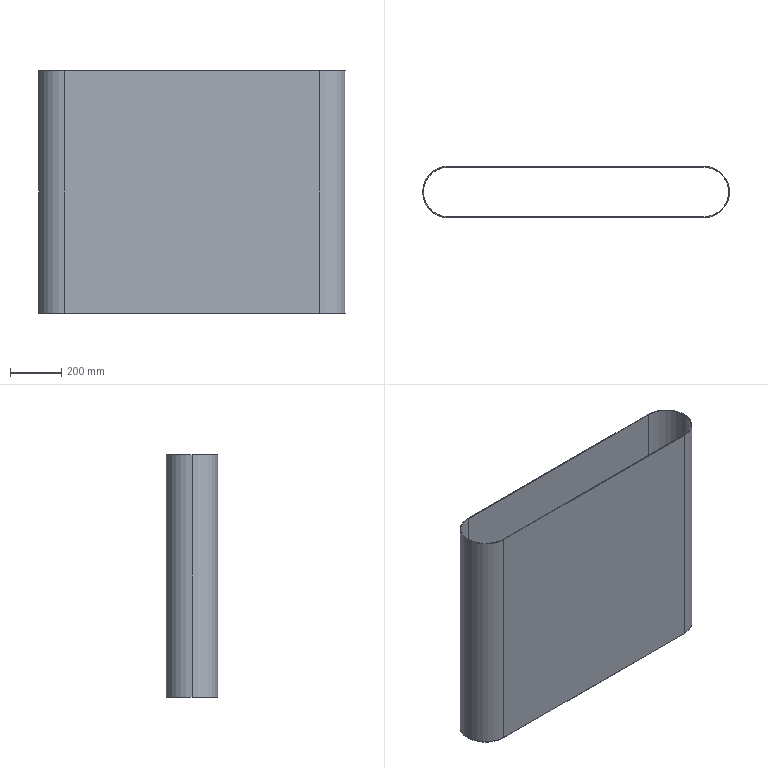Part | STEP file | Belt XG | 1 solid | 12 faces | box 1201 x 201 x 950 mm | volume 7472801 mm3 | cylinder 6 | plane 6 | commonest cylinder face diameters 195 x3 201 x3
STEP:
#1=CARTESIAN_POINT('',(0.,0.,0.));
#2=DIRECTION('',(0.,0.,1.));
#3=DIRECTION('',(1.,0.,0.));
#4=AXIS2_PLACEMENT_3D('',#1,#2,#3);
#5=CARTESIAN_POINT('',(-500.,97.5,475.));
#6=VERTEX_POINT('',#5);
#7=CARTESIAN_POINT('',(-500.,97.5,-475.));
#8=VERTEX_POINT('',#7);
#9=CARTESIAN_POINT('',(-500.,97.5,475.));
#10=DIRECTION('',(0.,0.,-1.));
#11=VECTOR('',#10,1.);
#12=LINE('',#9,#11);
#13=CARTESIAN_POINT('',(-500.,0.,475.));
#14=DIRECTION('',(0.,0.,-1.));
#15=DIRECTION('',(-1.,0.,0.));
#16=AXIS2_PLACEMENT_3D('',#13,#14,#15);
#17=CYLINDRICAL_SURFACE('',#16,97.5);
#18=CARTESIAN_POINT('',(1.571,0.));
#19=DIRECTION('',(0.,1.));
#20=VECTOR('',#19,1.);
#21=LINE('',#18,#20);
#22=(GEOMETRIC_REPRESENTATION_CONTEXT(2)PARAMETRIC_REPRESENTATION_CONTEXT()REPRESENTATION_CONTEXT('',''));
#23=DEFINITIONAL_REPRESENTATION('',(#21),#22);
#24=PCURVE('',#17,#23);
#25=CARTESIAN_POINT('',(-500.,97.5,475.));
#26=DIRECTION('',(0.,-1.,0.));
#27=DIRECTION('',(0.,0.,-1.));
#28=AXIS2_PLACEMENT_3D('',#25,#26,#27);
#29=PLANE('',#28);
#30=CARTESIAN_POINT('',(0.,0.));
#31=DIRECTION('',(1.,0.));
#32=VECTOR('',#31,1.);
#33=LINE('',#30,#32);
#34=(GEOMETRIC_REPRESENTATION_CONTEXT(2)PARAMETRIC_REPRESENTATION_CONTEXT()REPRESENTATION_CONTEXT('',''));
#35=DEFINITIONAL_REPRESENTATION('',(#33),#34);
#36=PCURVE('',#29,#35);
#37=SURFACE_CURVE('',#12,(#24,#36),.PCURVE_S1.);
#38=EDGE_CURVE('',#6,#8,#37,.T.);
#39=ORIENTED_EDGE('',*,*,#38,.T.);
#40=CARTESIAN_POINT('',(-597.5,0.,-475.));
#41=VERTEX_POINT('',#40);
#42=CARTESIAN_POINT('',(-500.,0.,-475.));
#43=DIRECTION('',(0.,0.,1.));
#44=DIRECTION('',(1.,0.,0.));
#45=AXIS2_PLACEMENT_3D('',#42,#43,#44);
#46=CIRCLE('',#45,97.5);
#47=CARTESIAN_POINT('',(3.142,950.));
#48=DIRECTION('',(-1.,0.));
#49=VECTOR('',#48,1.);
#50=LINE('',#47,#49);
#51=(GEOMETRIC_REPRESENTATION_CONTEXT(2)PARAMETRIC_REPRESENTATION_CONTEXT()REPRESENTATION_CONTEXT('',''));
#52=DEFINITIONAL_REPRESENTATION('',(#50),#51);
#53=PCURVE('',#17,#52);
#54=CARTESIAN_POINT('',(-500.,0.,-475.));
#55=DIRECTION('',(0.,0.,1.));
#56=DIRECTION('',(1.,0.,0.));
#57=AXIS2_PLACEMENT_3D('',#54,#55,#56);
#58=PLANE('',#57);
#59=CARTESIAN_POINT('',(0.,0.));
#60=DIRECTION('',(1.,0.));
#61=AXIS2_PLACEMENT_2D('',#59,#60);
#62=CIRCLE('',#61,97.5);
#63=(GEOMETRIC_REPRESENTATION_CONTEXT(2)PARAMETRIC_REPRESENTATION_CONTEXT()REPRESENTATION_CONTEXT('',''));
#64=DEFINITIONAL_REPRESENTATION('',(#62),#63);
#65=PCURVE('',#58,#64);
#66=SURFACE_CURVE('',#46,(#53,#65),.PCURVE_S1.);
#67=EDGE_CURVE('',#8,#41,#66,.T.);
#68=ORIENTED_EDGE('',*,*,#67,.T.);
#69=CARTESIAN_POINT('',(-597.5,0.,475.));
#70=VERTEX_POINT('',#69);
#71=CARTESIAN_POINT('',(-597.5,0.,475.));
#72=DIRECTION('',(0.,0.,-1.));
#73=VECTOR('',#72,1.);
#74=LINE('',#71,#73);
#75=CARTESIAN_POINT('',(0.,0.));
#76=DIRECTION('',(0.,1.));
#77=VECTOR('',#76,1.);
#78=LINE('',#75,#77);
#79=(GEOMETRIC_REPRESENTATION_CONTEXT(2)PARAMETRIC_REPRESENTATION_CONTEXT()REPRESENTATION_CONTEXT('',''));
#80=DEFINITIONAL_REPRESENTATION('',(#78),#79);
#81=PCURVE('',#17,#80);
#82=CARTESIAN_POINT('',(-500.,0.,475.));
#83=DIRECTION('',(0.,0.,-1.));
#84=DIRECTION('',(-1.,0.,0.));
#85=AXIS2_PLACEMENT_3D('',#82,#83,#84);
#86=CYLINDRICAL_SURFACE('',#85,97.5);
#87=CARTESIAN_POINT('',(6.283,0.));
#88=DIRECTION('',(0.,1.));
#89=VECTOR('',#88,1.);
#90=LINE('',#87,#89);
#91=(GEOMETRIC_REPRESENTATION_CONTEXT(2)PARAMETRIC_REPRESENTATION_CONTEXT()REPRESENTATION_CONTEXT('',''));
#92=DEFINITIONAL_REPRESENTATION('',(#90),#91);
#93=PCURVE('',#86,#92);
#94=SURFACE_CURVE('',#74,(#81,#93),.PCURVE_S1.);
#95=EDGE_CURVE('',#70,#41,#94,.T.);
#96=ORIENTED_EDGE('',*,*,#95,.F.);
#97=CARTESIAN_POINT('',(-500.,0.,475.));
#98=DIRECTION('',(0.,0.,1.));
#99=DIRECTION('',(1.,0.,0.));
#100=AXIS2_PLACEMENT_3D('',#97,#98,#99);
#101=CIRCLE('',#100,97.5);
#102=CARTESIAN_POINT('',(3.142,0.));
#103=DIRECTION('',(-1.,0.));
#104=VECTOR('',#103,1.);
#105=LINE('',#102,#104);
#106=(GEOMETRIC_REPRESENTATION_CONTEXT(2)PARAMETRIC_REPRESENTATION_CONTEXT()REPRESENTATION_CONTEXT('',''));
#107=DEFINITIONAL_REPRESENTATION('',(#105),#106);
#108=PCURVE('',#17,#107);
#109=CARTESIAN_POINT('',(-500.,0.,475.));
#110=DIRECTION('',(0.,0.,1.));
#111=DIRECTION('',(1.,0.,0.));
#112=AXIS2_PLACEMENT_3D('',#109,#110,#111);
#113=PLANE('',#112);
#114=CARTESIAN_POINT('',(0.,0.));
#115=DIRECTION('',(1.,0.));
#116=AXIS2_PLACEMENT_2D('',#114,#115);
#117=CIRCLE('',#116,97.5);
#118=(GEOMETRIC_REPRESENTATION_CONTEXT(2)PARAMETRIC_REPRESENTATION_CONTEXT()REPRESENTATION_CONTEXT('',''));
#119=DEFINITIONAL_REPRESENTATION('',(#117),#118);
#120=PCURVE('',#113,#119);
#121=SURFACE_CURVE('',#101,(#108,#120),.PCURVE_S1.);
#122=EDGE_CURVE('',#6,#70,#121,.T.);
#123=ORIENTED_EDGE('',*,*,#122,.F.);
#124=EDGE_LOOP('',(#39,#68,#96,#123));
#125=FACE_BOUND('',#124,.F.);
#126=ADVANCED_FACE('',(#125),#17,.F.);
#127=CARTESIAN_POINT('',(-600.5,0.,475.));
#128=VERTEX_POINT('',#127);
#129=CARTESIAN_POINT('',(-500.,-100.5,475.));
#130=VERTEX_POINT('',#129);
#131=CARTESIAN_POINT('',(-500.,0.,475.));
#132=DIRECTION('',(0.,0.,1.));
#133=DIRECTION('',(1.,0.,0.));
#134=AXIS2_PLACEMENT_3D('',#131,#132,#133);
#135=CIRCLE('',#134,100.5);
#136=CARTESIAN_POINT('',(-500.,0.,475.));
#137=DIRECTION('',(0.,0.,-1.));
#138=DIRECTION('',(-1.,0.,0.));
#139=AXIS2_PLACEMENT_3D('',#136,#137,#138);
#140=CYLINDRICAL_SURFACE('',#139,100.5);
#141=CARTESIAN_POINT('',(9.425,0.));
#142=DIRECTION('',(-1.,0.));
#143=VECTOR('',#142,1.);
#144=LINE('',#141,#143);
#145=(GEOMETRIC_REPRESENTATION_CONTEXT(2)PARAMETRIC_REPRESENTATION_CONTEXT()REPRESENTATION_CONTEXT('',''));
#146=DEFINITIONAL_REPRESENTATION('',(#144),#145);
#147=PCURVE('',#140,#146);
#148=CARTESIAN_POINT('',(0.,0.));
#149=DIRECTION('',(1.,0.));
#150=AXIS2_PLACEMENT_2D('',#148,#149);
#151=CIRCLE('',#150,100.5);
#152=(GEOMETRIC_REPRESENTATION_CONTEXT(2)PARAMETRIC_REPRESENTATION_CONTEXT()REPRESENTATION_CONTEXT('',''));
#153=DEFINITIONAL_REPRESENTATION('',(#151),#152);
#154=PCURVE('',#113,#153);
#155=SURFACE_CURVE('',#135,(#147,#154),.PCURVE_S1.);
#156=EDGE_CURVE('',#128,#130,#155,.T.);
#157=ORIENTED_EDGE('',*,*,#156,.F.);
#158=CARTESIAN_POINT('',(-600.5,0.,-475.));
#159=VERTEX_POINT('',#158);
#160=CARTESIAN_POINT('',(-600.5,0.,475.));
#161=DIRECTION('',(0.,0.,-1.));
#162=VECTOR('',#161,1.);
#163=LINE('',#160,#162);
#164=CARTESIAN_POINT('',(6.283,0.));
#165=DIRECTION('',(0.,1.));
#166=VECTOR('',#165,1.);
#167=LINE('',#164,#166);
#168=(GEOMETRIC_REPRESENTATION_CONTEXT(2)PARAMETRIC_REPRESENTATION_CONTEXT()REPRESENTATION_CONTEXT('',''));
#169=DEFINITIONAL_REPRESENTATION('',(#167),#168);
#170=PCURVE('',#140,#169);
#171=CARTESIAN_POINT('',(-500.,0.,475.));
#172=DIRECTION('',(0.,0.,-1.));
#173=DIRECTION('',(-1.,0.,0.));
#174=AXIS2_PLACEMENT_3D('',#171,#172,#173);
#175=CYLINDRICAL_SURFACE('',#174,100.5);
#176=CARTESIAN_POINT('',(0.,0.));
#177=DIRECTION('',(0.,1.));
#178=VECTOR('',#177,1.);
#179=LINE('',#176,#178);
#180=(GEOMETRIC_REPRESENTATION_CONTEXT(2)PARAMETRIC_REPRESENTATION_CONTEXT()REPRESENTATION_CONTEXT('',''));
#181=DEFINITIONAL_REPRESENTATION('',(#179),#180);
#182=PCURVE('',#175,#181);
#183=SURFACE_CURVE('',#163,(#170,#182),.PCURVE_S1.);
#184=EDGE_CURVE('',#128,#159,#183,.T.);
#185=ORIENTED_EDGE('',*,*,#184,.T.);
#186=CARTESIAN_POINT('',(-500.,-100.5,-475.));
#187=VERTEX_POINT('',#186);
#188=CARTESIAN_POINT('',(-500.,0.,-475.));
#189=DIRECTION('',(0.,0.,1.));
#190=DIRECTION('',(1.,0.,0.));
#191=AXIS2_PLACEMENT_3D('',#188,#189,#190);
#192=CIRCLE('',#191,100.5);
#193=CARTESIAN_POINT('',(9.425,950.));
#194=DIRECTION('',(-1.,0.));
#195=VECTOR('',#194,1.);
#196=LINE('',#193,#195);
#197=(GEOMETRIC_REPRESENTATION_CONTEXT(2)PARAMETRIC_REPRESENTATION_CONTEXT()REPRESENTATION_CONTEXT('',''));
#198=DEFINITIONAL_REPRESENTATION('',(#196),#197);
#199=PCURVE('',#140,#198);
#200=CARTESIAN_POINT('',(0.,0.));
#201=DIRECTION('',(1.,0.));
#202=AXIS2_PLACEMENT_2D('',#200,#201);
#203=CIRCLE('',#202,100.5);
#204=(GEOMETRIC_REPRESENTATION_CONTEXT(2)PARAMETRIC_REPRESENTATION_CONTEXT()REPRESENTATION_CONTEXT('',''));
#205=DEFINITIONAL_REPRESENTATION('',(#203),#204);
#206=PCURVE('',#58,#205);
#207=SURFACE_CURVE('',#192,(#199,#206),.PCURVE_S1.);
#208=EDGE_CURVE('',#159,#187,#207,.T.);
#209=ORIENTED_EDGE('',*,*,#208,.T.);
#210=CARTESIAN_POINT('',(-500.,-100.5,475.));
#211=DIRECTION('',(0.,0.,-1.));
#212=VECTOR('',#211,1.);
#213=LINE('',#210,#212);
#214=CARTESIAN_POINT('',(4.712,0.));
#215=DIRECTION('',(0.,1.));
#216=VECTOR('',#215,1.);
#217=LINE('',#214,#216);
#218=(GEOMETRIC_REPRESENTATION_CONTEXT(2)PARAMETRIC_REPRESENTATION_CONTEXT()REPRESENTATION_CONTEXT('',''));
#219=DEFINITIONAL_REPRESENTATION('',(#217),#218);
#220=PCURVE('',#140,#219);
#221=CARTESIAN_POINT('',(-500.,-100.5,475.));
#222=DIRECTION('',(0.,1.,0.));
#223=DIRECTION('',(0.,0.,1.));
#224=AXIS2_PLACEMENT_3D('',#221,#222,#223);
#225=PLANE('',#224);
#226=CARTESIAN_POINT('',(0.,0.));
#227=DIRECTION('',(-1.,0.));
#228=VECTOR('',#227,1.);
#229=LINE('',#226,#228);
#230=(GEOMETRIC_REPRESENTATION_CONTEXT(2)PARAMETRIC_REPRESENTATION_CONTEXT()REPRESENTATION_CONTEXT('',''));
#231=DEFINITIONAL_REPRESENTATION('',(#229),#230);
#232=PCURVE('',#225,#231);
#233=SURFACE_CURVE('',#213,(#220,#232),.PCURVE_S1.);
#234=EDGE_CURVE('',#130,#187,#233,.T.);
#235=ORIENTED_EDGE('',*,*,#234,.F.);
#236=EDGE_LOOP('',(#157,#185,#209,#235));
#237=FACE_BOUND('',#236,.T.);
#238=ADVANCED_FACE('',(#237),#140,.T.);
#239=CARTESIAN_POINT('',(-500.,100.5,475.));
#240=VERTEX_POINT('',#239);
#241=CARTESIAN_POINT('',(-500.,0.,475.));
#242=DIRECTION('',(0.,0.,1.));
#243=DIRECTION('',(1.,0.,0.));
#244=AXIS2_PLACEMENT_3D('',#241,#242,#243);
#245=CIRCLE('',#244,100.5);
#246=CARTESIAN_POINT('',(0.,0.));
#247=DIRECTION('',(1.,0.));
#248=AXIS2_PLACEMENT_2D('',#246,#247);
#249=CIRCLE('',#248,100.5);
#250=(GEOMETRIC_REPRESENTATION_CONTEXT(2)PARAMETRIC_REPRESENTATION_CONTEXT()REPRESENTATION_CONTEXT('',''));
#251=DEFINITIONAL_REPRESENTATION('',(#249),#250);
#252=PCURVE('',#113,#251);
#253=CARTESIAN_POINT('',(3.142,0.));
#254=DIRECTION('',(-1.,0.));
#255=VECTOR('',#254,1.);
#256=LINE('',#253,#255);
#257=(GEOMETRIC_REPRESENTATION_CONTEXT(2)PARAMETRIC_REPRESENTATION_CONTEXT()REPRESENTATION_CONTEXT('',''));
#258=DEFINITIONAL_REPRESENTATION('',(#256),#257);
#259=PCURVE('',#175,#258);
#260=SURFACE_CURVE('',#245,(#252,#259),.PCURVE_S1.);
#261=EDGE_CURVE('',#240,#128,#260,.T.);
#262=ORIENTED_EDGE('',*,*,#261,.T.);
#263=ORIENTED_EDGE('',*,*,#156,.T.);
#264=CARTESIAN_POINT('',(500.,-100.5,475.));
#265=VERTEX_POINT('',#264);
#266=CARTESIAN_POINT('',(-500.,-100.5,475.));
#267=DIRECTION('',(1.,0.,0.));
#268=VECTOR('',#267,1.);
#269=LINE('',#266,#268);
#270=CARTESIAN_POINT('',(0.,-100.5));
#271=DIRECTION('',(1.,0.));
#272=VECTOR('',#271,1.);
#273=LINE('',#270,#272);
#274=(GEOMETRIC_REPRESENTATION_CONTEXT(2)PARAMETRIC_REPRESENTATION_CONTEXT()REPRESENTATION_CONTEXT('',''));
#275=DEFINITIONAL_REPRESENTATION('',(#273),#274);
#276=PCURVE('',#113,#275);
#277=CARTESIAN_POINT('',(0.,0.));
#278=DIRECTION('',(0.,1.));
#279=VECTOR('',#278,1.);
#280=LINE('',#277,#279);
#281=(GEOMETRIC_REPRESENTATION_CONTEXT(2)PARAMETRIC_REPRESENTATION_CONTEXT()REPRESENTATION_CONTEXT('',''));
#282=DEFINITIONAL_REPRESENTATION('',(#280),#281);
#283=PCURVE('',#225,#282);
#284=SURFACE_CURVE('',#269,(#276,#283),.PCURVE_S1.);
#285=EDGE_CURVE('',#130,#265,#284,.T.);
#286=ORIENTED_EDGE('',*,*,#285,.T.);
#287=CARTESIAN_POINT('',(500.,100.5,475.));
#288=VERTEX_POINT('',#287);
#289=CARTESIAN_POINT('',(500.,0.,475.));
#290=DIRECTION('',(0.,0.,1.));
#291=DIRECTION('',(1.,0.,0.));
#292=AXIS2_PLACEMENT_3D('',#289,#290,#291);
#293=CIRCLE('',#292,100.5);
#294=CARTESIAN_POINT('',(1000.,0.));
#295=DIRECTION('',(1.,0.));
#296=AXIS2_PLACEMENT_2D('',#294,#295);
#297=CIRCLE('',#296,100.5);
#298=(GEOMETRIC_REPRESENTATION_CONTEXT(2)PARAMETRIC_REPRESENTATION_CONTEXT()REPRESENTATION_CONTEXT('',''));
#299=DEFINITIONAL_REPRESENTATION('',(#297),#298);
#300=PCURVE('',#113,#299);
#301=CARTESIAN_POINT('',(500.,0.,475.));
#302=DIRECTION('',(0.,0.,-1.));
#303=DIRECTION('',(-1.,0.,0.));
#304=AXIS2_PLACEMENT_3D('',#301,#302,#303);
#305=CYLINDRICAL_SURFACE('',#304,100.5);
#306=CARTESIAN_POINT('',(9.425,0.));
#307=DIRECTION('',(-1.,0.));
#308=VECTOR('',#307,1.);
#309=LINE('',#306,#308);
#310=(GEOMETRIC_REPRESENTATION_CONTEXT(2)PARAMETRIC_REPRESENTATION_CONTEXT()REPRESENTATION_CONTEXT('',''));
#311=DEFINITIONAL_REPRESENTATION('',(#309),#310);
#312=PCURVE('',#305,#311);
#313=SURFACE_CURVE('',#293,(#300,#312),.PCURVE_S1.);
#314=EDGE_CURVE('',#265,#288,#313,.T.);
#315=ORIENTED_EDGE('',*,*,#314,.T.);
#316=CARTESIAN_POINT('',(-500.,100.5,475.));
#317=DIRECTION('',(-1.,0.,0.));
#318=VECTOR('',#317,1.);
#319=LINE('',#316,#318);
#320=CARTESIAN_POINT('',(0.,100.5));
#321=DIRECTION('',(-1.,0.));
#322=VECTOR('',#321,1.);
#323=LINE('',#320,#322);
#324=(GEOMETRIC_REPRESENTATION_CONTEXT(2)PARAMETRIC_REPRESENTATION_CONTEXT()REPRESENTATION_CONTEXT('',''));
#325=DEFINITIONAL_REPRESENTATION('',(#323),#324);
#326=PCURVE('',#113,#325);
#327=CARTESIAN_POINT('',(-500.,100.5,475.));
#328=DIRECTION('',(0.,-1.,0.));
#329=DIRECTION('',(0.,0.,-1.));
#330=AXIS2_PLACEMENT_3D('',#327,#328,#329);
#331=PLANE('',#330);
#332=CARTESIAN_POINT('',(0.,0.));
#333=DIRECTION('',(0.,-1.));
#334=VECTOR('',#333,1.);
#335=LINE('',#332,#334);
#336=(GEOMETRIC_REPRESENTATION_CONTEXT(2)PARAMETRIC_REPRESENTATION_CONTEXT()REPRESENTATION_CONTEXT('',''));
#337=DEFINITIONAL_REPRESENTATION('',(#335),#336);
#338=PCURVE('',#331,#337);
#339=SURFACE_CURVE('',#319,(#326,#338),.PCURVE_S1.);
#340=EDGE_CURVE('',#288,#240,#339,.T.);
#341=ORIENTED_EDGE('',*,*,#340,.T.);
#342=EDGE_LOOP('',(#262,#263,#286,#315,#341));
#343=FACE_BOUND('',#342,.T.);
#344=CARTESIAN_POINT('',(-500.,-97.5,475.));
#345=VERTEX_POINT('',#344);
#346=CARTESIAN_POINT('',(500.,-97.5,475.));
#347=VERTEX_POINT('',#346);
#348=CARTESIAN_POINT('',(-500.,-97.5,475.));
#349=DIRECTION('',(1.,0.,0.));
#350=VECTOR('',#349,1.);
#351=LINE('',#348,#350);
#352=CARTESIAN_POINT('',(0.,-97.5));
#353=DIRECTION('',(1.,0.));
#354=VECTOR('',#353,1.);
#355=LINE('',#352,#354);
#356=(GEOMETRIC_REPRESENTATION_CONTEXT(2)PARAMETRIC_REPRESENTATION_CONTEXT()REPRESENTATION_CONTEXT('',''));
#357=DEFINITIONAL_REPRESENTATION('',(#355),#356);
#358=PCURVE('',#113,#357);
#359=CARTESIAN_POINT('',(-500.,-97.5,475.));
#360=DIRECTION('',(0.,1.,0.));
#361=DIRECTION('',(0.,0.,1.));
#362=AXIS2_PLACEMENT_3D('',#359,#360,#361);
#363=PLANE('',#362);
#364=CARTESIAN_POINT('',(0.,0.));
#365=DIRECTION('',(0.,1.));
#366=VECTOR('',#365,1.);
#367=LINE('',#364,#366);
#368=(GEOMETRIC_REPRESENTATION_CONTEXT(2)PARAMETRIC_REPRESENTATION_CONTEXT()REPRESENTATION_CONTEXT('',''));
#369=DEFINITIONAL_REPRESENTATION('',(#367),#368);
#370=PCURVE('',#363,#369);
#371=SURFACE_CURVE('',#351,(#358,#370),.PCURVE_S1.);
#372=EDGE_CURVE('',#345,#347,#371,.T.);
#373=ORIENTED_EDGE('',*,*,#372,.F.);
#374=CARTESIAN_POINT('',(-500.,0.,475.));
#375=DIRECTION('',(0.,0.,1.));
#376=DIRECTION('',(1.,0.,0.));
#377=AXIS2_PLACEMENT_3D('',#374,#375,#376);
#378=CIRCLE('',#377,97.5);
#379=CARTESIAN_POINT('',(0.,0.));
#380=DIRECTION('',(1.,0.));
#381=AXIS2_PLACEMENT_2D('',#379,#380);
#382=CIRCLE('',#381,97.5);
#383=(GEOMETRIC_REPRESENTATION_CONTEXT(2)PARAMETRIC_REPRESENTATION_CONTEXT()REPRESENTATION_CONTEXT('',''));
#384=DEFINITIONAL_REPRESENTATION('',(#382),#383);
#385=PCURVE('',#113,#384);
#386=CARTESIAN_POINT('',(9.425,0.));
#387=DIRECTION('',(-1.,0.));
#388=VECTOR('',#387,1.);
#389=LINE('',#386,#388);
#390=(GEOMETRIC_REPRESENTATION_CONTEXT(2)PARAMETRIC_REPRESENTATION_CONTEXT()REPRESENTATION_CONTEXT('',''));
#391=DEFINITIONAL_REPRESENTATION('',(#389),#390);
#392=PCURVE('',#86,#391);
#393=SURFACE_CURVE('',#378,(#385,#392),.PCURVE_S1.);
#394=EDGE_CURVE('',#70,#345,#393,.T.);
#395=ORIENTED_EDGE('',*,*,#394,.F.);
#396=ORIENTED_EDGE('',*,*,#122,.F.);
#397=CARTESIAN_POINT('',(500.,97.5,475.));
#398=VERTEX_POINT('',#397);
#399=CARTESIAN_POINT('',(-500.,97.5,475.));
#400=DIRECTION('',(-1.,0.,0.));
#401=VECTOR('',#400,1.);
#402=LINE('',#399,#401);
#403=CARTESIAN_POINT('',(0.,97.5));
#404=DIRECTION('',(-1.,0.));
#405=VECTOR('',#404,1.);
#406=LINE('',#403,#405);
#407=(GEOMETRIC_REPRESENTATION_CONTEXT(2)PARAMETRIC_REPRESENTATION_CONTEXT()REPRESENTATION_CONTEXT('',''));
#408=DEFINITIONAL_REPRESENTATION('',(#406),#407);
#409=PCURVE('',#113,#408);
#410=CARTESIAN_POINT('',(0.,0.));
#411=DIRECTION('',(0.,-1.));
#412=VECTOR('',#411,1.);
#413=LINE('',#410,#412);
#414=(GEOMETRIC_REPRESENTATION_CONTEXT(2)PARAMETRIC_REPRESENTATION_CONTEXT()REPRESENTATION_CONTEXT('',''));
#415=DEFINITIONAL_REPRESENTATION('',(#413),#414);
#416=PCURVE('',#29,#415);
#417=SURFACE_CURVE('',#402,(#409,#416),.PCURVE_S1.);
#418=EDGE_CURVE('',#398,#6,#417,.T.);
#419=ORIENTED_EDGE('',*,*,#418,.F.);
#420=CARTESIAN_POINT('',(500.,0.,475.));
#421=DIRECTION('',(0.,0.,1.));
#422=DIRECTION('',(1.,0.,0.));
#423=AXIS2_PLACEMENT_3D('',#420,#421,#422);
#424=CIRCLE('',#423,97.5);
#425=CARTESIAN_POINT('',(1000.,0.));
#426=DIRECTION('',(1.,0.));
#427=AXIS2_PLACEMENT_2D('',#425,#426);
#428=CIRCLE('',#427,97.5);
#429=(GEOMETRIC_REPRESENTATION_CONTEXT(2)PARAMETRIC_REPRESENTATION_CONTEXT()REPRESENTATION_CONTEXT('',''));
#430=DEFINITIONAL_REPRESENTATION('',(#428),#429);
#431=PCURVE('',#113,#430);
#432=CARTESIAN_POINT('',(500.,0.,475.));
#433=DIRECTION('',(0.,0.,-1.));
#434=DIRECTION('',(-1.,0.,0.));
#435=AXIS2_PLACEMENT_3D('',#432,#433,#434);
#436=CYLINDRICAL_SURFACE('',#435,97.5);
#437=CARTESIAN_POINT('',(9.425,0.));
#438=DIRECTION('',(-1.,0.));
#439=VECTOR('',#438,1.);
#440=LINE('',#437,#439);
#441=(GEOMETRIC_REPRESENTATION_CONTEXT(2)PARAMETRIC_REPRESENTATION_CONTEXT()REPRESENTATION_CONTEXT('',''));
#442=DEFINITIONAL_REPRESENTATION('',(#440),#441);
#443=PCURVE('',#436,#442);
#444=SURFACE_CURVE('',#424,(#431,#443),.PCURVE_S1.);
#445=EDGE_CURVE('',#347,#398,#444,.T.);
#446=ORIENTED_EDGE('',*,*,#445,.F.);
#447=EDGE_LOOP('',(#373,#395,#396,#419,#446));
#448=FACE_BOUND('',#447,.T.);
#449=ADVANCED_FACE('',(#343,#448),#113,.T.);
#450=CARTESIAN_POINT('',(-500.,100.5,-475.));
#451=VERTEX_POINT('',#450);
#452=CARTESIAN_POINT('',(-500.,0.,-475.));
#453=DIRECTION('',(0.,0.,1.));
#454=DIRECTION('',(1.,0.,0.));
#455=AXIS2_PLACEMENT_3D('',#452,#453,#454);
#456=CIRCLE('',#455,100.5);
#457=CARTESIAN_POINT('',(0.,0.));
#458=DIRECTION('',(1.,0.));
#459=AXIS2_PLACEMENT_2D('',#457,#458);
#460=CIRCLE('',#459,100.5);
#461=(GEOMETRIC_REPRESENTATION_CONTEXT(2)PARAMETRIC_REPRESENTATION_CONTEXT()REPRESENTATION_CONTEXT('',''));
#462=DEFINITIONAL_REPRESENTATION('',(#460),#461);
#463=PCURVE('',#58,#462);
#464=CARTESIAN_POINT('',(3.142,950.));
#465=DIRECTION('',(-1.,0.));
#466=VECTOR('',#465,1.);
#467=LINE('',#464,#466);
#468=(GEOMETRIC_REPRESENTATION_CONTEXT(2)PARAMETRIC_REPRESENTATION_CONTEXT()REPRESENTATION_CONTEXT('',''));
#469=DEFINITIONAL_REPRESENTATION('',(#467),#468);
#470=PCURVE('',#175,#469);
#471=SURFACE_CURVE('',#456,(#463,#470),.PCURVE_S1.);
#472=EDGE_CURVE('',#451,#159,#471,.T.);
#473=ORIENTED_EDGE('',*,*,#472,.F.);
#474=CARTESIAN_POINT('',(500.,100.5,-475.));
#475=VERTEX_POINT('',#474);
#476=CARTESIAN_POINT('',(-500.,100.5,-475.));
#477=DIRECTION('',(-1.,0.,0.));
#478=VECTOR('',#477,1.);
#479=LINE('',#476,#478);
#480=CARTESIAN_POINT('',(0.,100.5));
#481=DIRECTION('',(-1.,0.));
#482=VECTOR('',#481,1.);
#483=LINE('',#480,#482);
#484=(GEOMETRIC_REPRESENTATION_CONTEXT(2)PARAMETRIC_REPRESENTATION_CONTEXT()REPRESENTATION_CONTEXT('',''));
#485=DEFINITIONAL_REPRESENTATION('',(#483),#484);
#486=PCURVE('',#58,#485);
#487=CARTESIAN_POINT('',(950.,0.));
#488=DIRECTION('',(0.,-1.));
#489=VECTOR('',#488,1.);
#490=LINE('',#487,#489);
#491=(GEOMETRIC_REPRESENTATION_CONTEXT(2)PARAMETRIC_REPRESENTATION_CONTEXT()REPRESENTATION_CONTEXT('',''));
#492=DEFINITIONAL_REPRESENTATION('',(#490),#491);
#493=PCURVE('',#331,#492);
#494=SURFACE_CURVE('',#479,(#486,#493),.PCURVE_S1.);
#495=EDGE_CURVE('',#475,#451,#494,.T.);
#496=ORIENTED_EDGE('',*,*,#495,.F.);
#497=CARTESIAN_POINT('',(500.,-100.5,-475.));
#498=VERTEX_POINT('',#497);
#499=CARTESIAN_POINT('',(500.,0.,-475.));
#500=DIRECTION('',(0.,0.,1.));
#501=DIRECTION('',(1.,0.,0.));
#502=AXIS2_PLACEMENT_3D('',#499,#500,#501);
#503=CIRCLE('',#502,100.5);
#504=CARTESIAN_POINT('',(1000.,0.));
#505=DIRECTION('',(1.,0.));
#506=AXIS2_PLACEMENT_2D('',#504,#505);
#507=CIRCLE('',#506,100.5);
#508=(GEOMETRIC_REPRESENTATION_CONTEXT(2)PARAMETRIC_REPRESENTATION_CONTEXT()REPRESENTATION_CONTEXT('',''));
#509=DEFINITIONAL_REPRESENTATION('',(#507),#508);
#510=PCURVE('',#58,#509);
#511=CARTESIAN_POINT('',(9.425,950.));
#512=DIRECTION('',(-1.,0.));
#513=VECTOR('',#512,1.);
#514=LINE('',#511,#513);
#515=(GEOMETRIC_REPRESENTATION_CONTEXT(2)PARAMETRIC_REPRESENTATION_CONTEXT()REPRESENTATION_CONTEXT('',''));
#516=DEFINITIONAL_REPRESENTATION('',(#514),#515);
#517=PCURVE('',#305,#516);
#518=SURFACE_CURVE('',#503,(#510,#517),.PCURVE_S1.);
#519=EDGE_CURVE('',#498,#475,#518,.T.);
#520=ORIENTED_EDGE('',*,*,#519,.F.);
#521=CARTESIAN_POINT('',(-500.,-100.5,-475.));
#522=DIRECTION('',(1.,0.,0.));
#523=VECTOR('',#522,1.);
#524=LINE('',#521,#523);
#525=CARTESIAN_POINT('',(0.,-100.5));
#526=DIRECTION('',(1.,0.));
#527=VECTOR('',#526,1.);
#528=LINE('',#525,#527);
#529=(GEOMETRIC_REPRESENTATION_CONTEXT(2)PARAMETRIC_REPRESENTATION_CONTEXT()REPRESENTATION_CONTEXT('',''));
#530=DEFINITIONAL_REPRESENTATION('',(#528),#529);
#531=PCURVE('',#58,#530);
#532=CARTESIAN_POINT('',(-950.,0.));
#533=DIRECTION('',(0.,1.));
#534=VECTOR('',#533,1.);
#535=LINE('',#532,#534);
#536=(GEOMETRIC_REPRESENTATION_CONTEXT(2)PARAMETRIC_REPRESENTATION_CONTEXT()REPRESENTATION_CONTEXT('',''));
#537=DEFINITIONAL_REPRESENTATION('',(#535),#536);
#538=PCURVE('',#225,#537);
#539=SURFACE_CURVE('',#524,(#531,#538),.PCURVE_S1.);
#540=EDGE_CURVE('',#187,#498,#539,.T.);
#541=ORIENTED_EDGE('',*,*,#540,.F.);
#542=ORIENTED_EDGE('',*,*,#208,.F.);
#543=EDGE_LOOP('',(#473,#496,#520,#541,#542));
#544=FACE_BOUND('',#543,.T.);
#545=ORIENTED_EDGE('',*,*,#67,.T.);
#546=CARTESIAN_POINT('',(-500.,-97.5,-475.));
#547=VERTEX_POINT('',#546);
#548=CARTESIAN_POINT('',(-500.,0.,-475.));
#549=DIRECTION('',(0.,0.,1.));
#550=DIRECTION('',(1.,0.,0.));
#551=AXIS2_PLACEMENT_3D('',#548,#549,#550);
#552=CIRCLE('',#551,97.5);
#553=CARTESIAN_POINT('',(0.,0.));
#554=DIRECTION('',(1.,0.));
#555=AXIS2_PLACEMENT_2D('',#553,#554);
#556=CIRCLE('',#555,97.5);
#557=(GEOMETRIC_REPRESENTATION_CONTEXT(2)PARAMETRIC_REPRESENTATION_CONTEXT()REPRESENTATION_CONTEXT('',''));
#558=DEFINITIONAL_REPRESENTATION('',(#556),#557);
#559=PCURVE('',#58,#558);
#560=CARTESIAN_POINT('',(9.425,950.));
#561=DIRECTION('',(-1.,0.));
#562=VECTOR('',#561,1.);
#563=LINE('',#560,#562);
#564=(GEOMETRIC_REPRESENTATION_CONTEXT(2)PARAMETRIC_REPRESENTATION_CONTEXT()REPRESENTATION_CONTEXT('',''));
#565=DEFINITIONAL_REPRESENTATION('',(#563),#564);
#566=PCURVE('',#86,#565);
#567=SURFACE_CURVE('',#552,(#559,#566),.PCURVE_S1.);
#568=EDGE_CURVE('',#41,#547,#567,.T.);
#569=ORIENTED_EDGE('',*,*,#568,.T.);
#570=CARTESIAN_POINT('',(500.,-97.5,-475.));
#571=VERTEX_POINT('',#570);
#572=CARTESIAN_POINT('',(-500.,-97.5,-475.));
#573=DIRECTION('',(1.,0.,0.));
#574=VECTOR('',#573,1.);
#575=LINE('',#572,#574);
#576=CARTESIAN_POINT('',(0.,-97.5));
#577=DIRECTION('',(1.,0.));
#578=VECTOR('',#577,1.);
#579=LINE('',#576,#578);
#580=(GEOMETRIC_REPRESENTATION_CONTEXT(2)PARAMETRIC_REPRESENTATION_CONTEXT()REPRESENTATION_CONTEXT('',''));
#581=DEFINITIONAL_REPRESENTATION('',(#579),#580);
#582=PCURVE('',#58,#581);
#583=CARTESIAN_POINT('',(-950.,0.));
#584=DIRECTION('',(0.,1.));
#585=VECTOR('',#584,1.);
#586=LINE('',#583,#585);
#587=(GEOMETRIC_REPRESENTATION_CONTEXT(2)PARAMETRIC_REPRESENTATION_CONTEXT()REPRESENTATION_CONTEXT('',''));
#588=DEFINITIONAL_REPRESENTATION('',(#586),#587);
#589=PCURVE('',#363,#588);
#590=SURFACE_CURVE('',#575,(#582,#589),.PCURVE_S1.);
#591=EDGE_CURVE('',#547,#571,#590,.T.);
#592=ORIENTED_EDGE('',*,*,#591,.T.);
#593=CARTESIAN_POINT('',(500.,97.5,-475.));
#594=VERTEX_POINT('',#593);
#595=CARTESIAN_POINT('',(500.,0.,-475.));
#596=DIRECTION('',(0.,0.,1.));
#597=DIRECTION('',(1.,0.,0.));
#598=AXIS2_PLACEMENT_3D('',#595,#596,#597);
#599=CIRCLE('',#598,97.5);
#600=CARTESIAN_POINT('',(1000.,0.));
#601=DIRECTION('',(1.,0.));
#602=AXIS2_PLACEMENT_2D('',#600,#601);
#603=CIRCLE('',#602,97.5);
#604=(GEOMETRIC_REPRESENTATION_CONTEXT(2)PARAMETRIC_REPRESENTATION_CONTEXT()REPRESENTATION_CONTEXT('',''));
#605=DEFINITIONAL_REPRESENTATION('',(#603),#604);
#606=PCURVE('',#58,#605);
#607=CARTESIAN_POINT('',(9.425,950.));
#608=DIRECTION('',(-1.,0.));
#609=VECTOR('',#608,1.);
#610=LINE('',#607,#609);
#611=(GEOMETRIC_REPRESENTATION_CONTEXT(2)PARAMETRIC_REPRESENTATION_CONTEXT()REPRESENTATION_CONTEXT('',''));
#612=DEFINITIONAL_REPRESENTATION('',(#610),#611);
#613=PCURVE('',#436,#612);
#614=SURFACE_CURVE('',#599,(#606,#613),.PCURVE_S1.);
#615=EDGE_CURVE('',#571,#594,#614,.T.);
#616=ORIENTED_EDGE('',*,*,#615,.T.);
#617=CARTESIAN_POINT('',(-500.,97.5,-475.));
#618=DIRECTION('',(-1.,0.,0.));
#619=VECTOR('',#618,1.);
#620=LINE('',#617,#619);
#621=CARTESIAN_POINT('',(0.,97.5));
#622=DIRECTION('',(-1.,0.));
#623=VECTOR('',#622,1.);
#624=LINE('',#621,#623);
#625=(GEOMETRIC_REPRESENTATION_CONTEXT(2)PARAMETRIC_REPRESENTATION_CONTEXT()REPRESENTATION_CONTEXT('',''));
#626=DEFINITIONAL_REPRESENTATION('',(#624),#625);
#627=PCURVE('',#58,#626);
#628=CARTESIAN_POINT('',(950.,0.));
#629=DIRECTION('',(0.,-1.));
#630=VECTOR('',#629,1.);
#631=LINE('',#628,#630);
#632=(GEOMETRIC_REPRESENTATION_CONTEXT(2)PARAMETRIC_REPRESENTATION_CONTEXT()REPRESENTATION_CONTEXT('',''));
#633=DEFINITIONAL_REPRESENTATION('',(#631),#632);
#634=PCURVE('',#29,#633);
#635=SURFACE_CURVE('',#620,(#627,#634),.PCURVE_S1.);
#636=EDGE_CURVE('',#594,#8,#635,.T.);
#637=ORIENTED_EDGE('',*,*,#636,.T.);
#638=EDGE_LOOP('',(#545,#569,#592,#616,#637));
#639=FACE_BOUND('',#638,.T.);
#640=ADVANCED_FACE('',(#544,#639),#58,.F.);
#641=ORIENTED_EDGE('',*,*,#184,.F.);
#642=ORIENTED_EDGE('',*,*,#261,.F.);
#643=CARTESIAN_POINT('',(-500.,100.5,475.));
#644=DIRECTION('',(0.,0.,-1.));
#645=VECTOR('',#644,1.);
#646=LINE('',#643,#645);
#647=CARTESIAN_POINT('',(1.571,0.));
#648=DIRECTION('',(0.,1.));
#649=VECTOR('',#648,1.);
#650=LINE('',#647,#649);
#651=(GEOMETRIC_REPRESENTATION_CONTEXT(2)PARAMETRIC_REPRESENTATION_CONTEXT()REPRESENTATION_CONTEXT('',''));
#652=DEFINITIONAL_REPRESENTATION('',(#650),#651);
#653=PCURVE('',#175,#652);
#654=CARTESIAN_POINT('',(0.,0.));
#655=DIRECTION('',(1.,0.));
#656=VECTOR('',#655,1.);
#657=LINE('',#654,#656);
#658=(GEOMETRIC_REPRESENTATION_CONTEXT(2)PARAMETRIC_REPRESENTATION_CONTEXT()REPRESENTATION_CONTEXT('',''));
#659=DEFINITIONAL_REPRESENTATION('',(#657),#658);
#660=PCURVE('',#331,#659);
#661=SURFACE_CURVE('',#646,(#653,#660),.PCURVE_S1.);
#662=EDGE_CURVE('',#240,#451,#661,.T.);
#663=ORIENTED_EDGE('',*,*,#662,.T.);
#664=ORIENTED_EDGE('',*,*,#472,.T.);
#665=EDGE_LOOP('',(#641,#642,#663,#664));
#666=FACE_BOUND('',#665,.T.);
#667=ADVANCED_FACE('',(#666),#175,.T.);
#668=ORIENTED_EDGE('',*,*,#540,.T.);
#669=CARTESIAN_POINT('',(500.,-100.5,475.));
#670=DIRECTION('',(0.,0.,-1.));
#671=VECTOR('',#670,1.);
#672=LINE('',#669,#671);
#673=CARTESIAN_POINT('',(0.,1000.));
#674=DIRECTION('',(-1.,0.));
#675=VECTOR('',#674,1.);
#676=LINE('',#673,#675);
#677=(GEOMETRIC_REPRESENTATION_CONTEXT(2)PARAMETRIC_REPRESENTATION_CONTEXT()REPRESENTATION_CONTEXT('',''));
#678=DEFINITIONAL_REPRESENTATION('',(#676),#677);
#679=PCURVE('',#225,#678);
#680=CARTESIAN_POINT('',(4.712,0.));
#681=DIRECTION('',(0.,1.));
#682=VECTOR('',#681,1.);
#683=LINE('',#680,#682);
#684=(GEOMETRIC_REPRESENTATION_CONTEXT(2)PARAMETRIC_REPRESENTATION_CONTEXT()REPRESENTATION_CONTEXT('',''));
#685=DEFINITIONAL_REPRESENTATION('',(#683),#684);
#686=PCURVE('',#305,#685);
#687=SURFACE_CURVE('',#672,(#679,#686),.PCURVE_S1.);
#688=EDGE_CURVE('',#265,#498,#687,.T.);
#689=ORIENTED_EDGE('',*,*,#688,.F.);
#690=ORIENTED_EDGE('',*,*,#285,.F.);
#691=ORIENTED_EDGE('',*,*,#234,.T.);
#692=EDGE_LOOP('',(#668,#689,#690,#691));
#693=FACE_BOUND('',#692,.T.);
#694=ADVANCED_FACE('',(#693),#225,.F.);
#695=ORIENTED_EDGE('',*,*,#519,.T.);
#696=CARTESIAN_POINT('',(500.,100.5,475.));
#697=DIRECTION('',(0.,0.,-1.));
#698=VECTOR('',#697,1.);
#699=LINE('',#696,#698);
#700=CARTESIAN_POINT('',(1.571,0.));
#701=DIRECTION('',(0.,1.));
#702=VECTOR('',#701,1.);
#703=LINE('',#700,#702);
#704=(GEOMETRIC_REPRESENTATION_CONTEXT(2)PARAMETRIC_REPRESENTATION_CONTEXT()REPRESENTATION_CONTEXT('',''));
#705=DEFINITIONAL_REPRESENTATION('',(#703),#704);
#706=PCURVE('',#305,#705);
#707=CARTESIAN_POINT('',(0.,1000.));
#708=DIRECTION('',(1.,0.));
#709=VECTOR('',#708,1.);
#710=LINE('',#707,#709);
#711=(GEOMETRIC_REPRESENTATION_CONTEXT(2)PARAMETRIC_REPRESENTATION_CONTEXT()REPRESENTATION_CONTEXT('',''));
#712=DEFINITIONAL_REPRESENTATION('',(#710),#711);
#713=PCURVE('',#331,#712);
#714=SURFACE_CURVE('',#699,(#706,#713),.PCURVE_S1.);
#715=EDGE_CURVE('',#288,#475,#714,.T.);
#716=ORIENTED_EDGE('',*,*,#715,.F.);
#717=ORIENTED_EDGE('',*,*,#314,.F.);
#718=ORIENTED_EDGE('',*,*,#688,.T.);
#719=EDGE_LOOP('',(#695,#716,#717,#718));
#720=FACE_BOUND('',#719,.T.);
#721=ADVANCED_FACE('',(#720),#305,.T.);
#722=ORIENTED_EDGE('',*,*,#495,.T.);
#723=ORIENTED_EDGE('',*,*,#662,.F.);
#724=ORIENTED_EDGE('',*,*,#340,.F.);
#725=ORIENTED_EDGE('',*,*,#715,.T.);
#726=EDGE_LOOP('',(#722,#723,#724,#725));
#727=FACE_BOUND('',#726,.T.);
#728=ADVANCED_FACE('',(#727),#331,.F.);
#729=ORIENTED_EDGE('',*,*,#568,.T.);
#730=CARTESIAN_POINT('',(-500.,-97.5,475.));
#731=DIRECTION('',(0.,0.,-1.));
#732=VECTOR('',#731,1.);
#733=LINE('',#730,#732);
#734=CARTESIAN_POINT('',(4.712,0.));
#735=DIRECTION('',(0.,1.));
#736=VECTOR('',#735,1.);
#737=LINE('',#734,#736);
#738=(GEOMETRIC_REPRESENTATION_CONTEXT(2)PARAMETRIC_REPRESENTATION_CONTEXT()REPRESENTATION_CONTEXT('',''));
#739=DEFINITIONAL_REPRESENTATION('',(#737),#738);
#740=PCURVE('',#86,#739);
#741=CARTESIAN_POINT('',(0.,0.));
#742=DIRECTION('',(-1.,0.));
#743=VECTOR('',#742,1.);
#744=LINE('',#741,#743);
#745=(GEOMETRIC_REPRESENTATION_CONTEXT(2)PARAMETRIC_REPRESENTATION_CONTEXT()REPRESENTATION_CONTEXT('',''));
#746=DEFINITIONAL_REPRESENTATION('',(#744),#745);
#747=PCURVE('',#363,#746);
#748=SURFACE_CURVE('',#733,(#740,#747),.PCURVE_S1.);
#749=EDGE_CURVE('',#345,#547,#748,.T.);
#750=ORIENTED_EDGE('',*,*,#749,.F.);
#751=ORIENTED_EDGE('',*,*,#394,.F.);
#752=ORIENTED_EDGE('',*,*,#95,.T.);
#753=EDGE_LOOP('',(#729,#750,#751,#752));
#754=FACE_BOUND('',#753,.F.);
#755=ADVANCED_FACE('',(#754),#86,.F.);
#756=ORIENTED_EDGE('',*,*,#591,.F.);
#757=ORIENTED_EDGE('',*,*,#749,.F.);
#758=ORIENTED_EDGE('',*,*,#372,.T.);
#759=CARTESIAN_POINT('',(500.,-97.5,475.));
#760=DIRECTION('',(0.,0.,-1.));
#761=VECTOR('',#760,1.);
#762=LINE('',#759,#761);
#763=CARTESIAN_POINT('',(0.,1000.));
#764=DIRECTION('',(-1.,0.));
#765=VECTOR('',#764,1.);
#766=LINE('',#763,#765);
#767=(GEOMETRIC_REPRESENTATION_CONTEXT(2)PARAMETRIC_REPRESENTATION_CONTEXT()REPRESENTATION_CONTEXT('',''));
#768=DEFINITIONAL_REPRESENTATION('',(#766),#767);
#769=PCURVE('',#363,#768);
#770=CARTESIAN_POINT('',(4.712,0.));
#771=DIRECTION('',(0.,1.));
#772=VECTOR('',#771,1.);
#773=LINE('',#770,#772);
#774=(GEOMETRIC_REPRESENTATION_CONTEXT(2)PARAMETRIC_REPRESENTATION_CONTEXT()REPRESENTATION_CONTEXT('',''));
#775=DEFINITIONAL_REPRESENTATION('',(#773),#774);
#776=PCURVE('',#436,#775);
#777=SURFACE_CURVE('',#762,(#769,#776),.PCURVE_S1.);
#778=EDGE_CURVE('',#347,#571,#777,.T.);
#779=ORIENTED_EDGE('',*,*,#778,.T.);
#780=EDGE_LOOP('',(#756,#757,#758,#779));
#781=FACE_BOUND('',#780,.T.);
#782=ADVANCED_FACE('',(#781),#363,.T.);
#783=CARTESIAN_POINT('',(500.,97.5,475.));
#784=DIRECTION('',(0.,0.,-1.));
#785=VECTOR('',#784,1.);
#786=LINE('',#783,#785);
#787=CARTESIAN_POINT('',(1.571,0.));
#788=DIRECTION('',(0.,1.));
#789=VECTOR('',#788,1.);
#790=LINE('',#787,#789);
#791=(GEOMETRIC_REPRESENTATION_CONTEXT(2)PARAMETRIC_REPRESENTATION_CONTEXT()REPRESENTATION_CONTEXT('',''));
#792=DEFINITIONAL_REPRESENTATION('',(#790),#791);
#793=PCURVE('',#436,#792);
#794=CARTESIAN_POINT('',(0.,1000.));
#795=DIRECTION('',(1.,0.));
#796=VECTOR('',#795,1.);
#797=LINE('',#794,#796);
#798=(GEOMETRIC_REPRESENTATION_CONTEXT(2)PARAMETRIC_REPRESENTATION_CONTEXT()REPRESENTATION_CONTEXT('',''));
#799=DEFINITIONAL_REPRESENTATION('',(#797),#798);
#800=PCURVE('',#29,#799);
#801=SURFACE_CURVE('',#786,(#793,#800),.PCURVE_S1.);
#802=EDGE_CURVE('',#398,#594,#801,.T.);
#803=ORIENTED_EDGE('',*,*,#802,.F.);
#804=ORIENTED_EDGE('',*,*,#445,.F.);
#805=ORIENTED_EDGE('',*,*,#778,.T.);
#806=ORIENTED_EDGE('',*,*,#615,.T.);
#807=EDGE_LOOP('',(#803,#804,#805,#806));
#808=FACE_BOUND('',#807,.F.);
#809=ADVANCED_FACE('',(#808),#436,.F.);
#810=ORIENTED_EDGE('',*,*,#636,.F.);
#811=ORIENTED_EDGE('',*,*,#802,.F.);
#812=ORIENTED_EDGE('',*,*,#418,.T.);
#813=ORIENTED_EDGE('',*,*,#38,.T.);
#814=EDGE_LOOP('',(#810,#811,#812,#813));
#815=FACE_BOUND('',#814,.T.);
#816=ADVANCED_FACE('',(#815),#29,.T.);
#817=CLOSED_SHELL('',(#126,#238,#449,#640,#667,#694,#721,#728,#755,#782,#809,#816));
#818=MANIFOLD_SOLID_BREP('',#817);
#819=(LENGTH_UNIT()NAMED_UNIT(*)SI_UNIT(.MILLI.,.METRE.));
#820=UNCERTAINTY_MEASURE_WITH_UNIT(LENGTH_MEASURE(0.0000001),#819,'','');
#821=(NAMED_UNIT(*)PLANE_ANGLE_UNIT()SI_UNIT($,.RADIAN.));
#822=(NAMED_UNIT(*)SI_UNIT($,.STERADIAN.)SOLID_ANGLE_UNIT());
#823=(GEOMETRIC_REPRESENTATION_CONTEXT(3)GLOBAL_UNCERTAINTY_ASSIGNED_CONTEXT((#820))GLOBAL_UNIT_ASSIGNED_CONTEXT((#819,#821,#822))REPRESENTATION_CONTEXT('',''));
#824=ADVANCED_BREP_SHAPE_REPRESENTATION('',(#4,#818),#823);